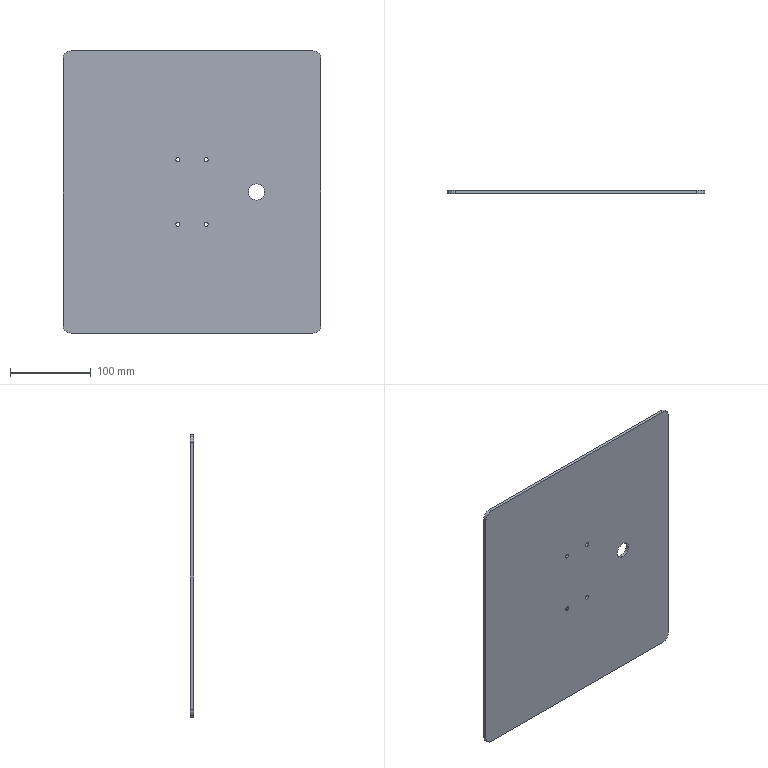Part | SolidWorks | features Extrusion 1, Fillet 1, HoleWzd 1, ICE 1 | 1 solid | 20 faces | box 320 x 4 x 350 mm | volume 446060 mm3 | cylinder 14 | plane 6 | commonest cylinder face diameters 5.2 x8 20 x6
STEP:
#1=CARTESIAN_POINT('',(80.,0.,-10.));
#2=VERTEX_POINT('',#1);
#3=CARTESIAN_POINT('',(80.,0.,10.));
#4=VERTEX_POINT('',#3);
#5=CARTESIAN_POINT('',(80.,0.,0.));
#6=DIRECTION('',(0.,1.,0.));
#7=DIRECTION('',(0.,0.,1.));
#8=AXIS2_PLACEMENT_3D('',#5,#6,#7);
#9=CIRCLE('',#8,10.);
#10=EDGE_CURVE('',#2,#4,#9,.T.);
#11=ORIENTED_EDGE('',*,*,#10,.F.);
#12=CARTESIAN_POINT('',(80.,4.,-10.));
#13=VERTEX_POINT('',#12);
#14=CARTESIAN_POINT('',(80.,0.,-10.));
#15=DIRECTION('',(0.,1.,0.));
#16=VECTOR('',#15,1000.);
#17=LINE('',#14,#16);
#18=EDGE_CURVE('',#2,#13,#17,.T.);
#19=ORIENTED_EDGE('',*,*,#18,.T.);
#20=CARTESIAN_POINT('',(80.,4.,10.));
#21=VERTEX_POINT('',#20);
#22=CARTESIAN_POINT('',(80.,4.,0.));
#23=DIRECTION('',(0.,1.,0.));
#24=DIRECTION('',(0.,0.,1.));
#25=AXIS2_PLACEMENT_3D('',#22,#23,#24);
#26=CIRCLE('',#25,10.);
#27=EDGE_CURVE('',#13,#21,#26,.T.);
#28=ORIENTED_EDGE('',*,*,#27,.T.);
#29=CARTESIAN_POINT('',(80.,0.,10.));
#30=DIRECTION('',(0.,1.,0.));
#31=VECTOR('',#30,1000.);
#32=LINE('',#29,#31);
#33=EDGE_CURVE('',#4,#21,#32,.T.);
#34=ORIENTED_EDGE('',*,*,#33,.F.);
#35=EDGE_LOOP('',(#11,#19,#28,#34));
#36=FACE_OUTER_BOUND('',#35,.T.);
#37=CARTESIAN_POINT('',(80.,0.,0.));
#38=DIRECTION('',(0.,1.,0.));
#39=DIRECTION('',(0.,0.,1.));
#40=AXIS2_PLACEMENT_3D('',#37,#38,#39);
#41=CYLINDRICAL_SURFACE('',#40,10.);
#42=ADVANCED_FACE('',(#36),#41,.F.);
#43=CARTESIAN_POINT('',(-17.5,0.,-42.6));
#44=VERTEX_POINT('',#43);
#45=CARTESIAN_POINT('',(-17.5,0.,-37.4));
#46=VERTEX_POINT('',#45);
#47=CARTESIAN_POINT('',(-17.5,0.,-40.));
#48=DIRECTION('',(0.,1.,0.));
#49=DIRECTION('',(0.,0.,1.));
#50=AXIS2_PLACEMENT_3D('',#47,#48,#49);
#51=CIRCLE('',#50,2.6);
#52=EDGE_CURVE('',#44,#46,#51,.T.);
#53=ORIENTED_EDGE('',*,*,#52,.F.);
#54=CARTESIAN_POINT('',(-17.5,4.,-42.6));
#55=VERTEX_POINT('',#54);
#56=CARTESIAN_POINT('',(-17.5,4.,-42.6));
#57=DIRECTION('',(0.,1.,0.));
#58=VECTOR('',#57,1000.);
#59=LINE('',#56,#58);
#60=EDGE_CURVE('',#44,#55,#59,.T.);
#61=ORIENTED_EDGE('',*,*,#60,.T.);
#62=CARTESIAN_POINT('',(-17.5,4.,-37.4));
#63=VERTEX_POINT('',#62);
#64=CARTESIAN_POINT('',(-17.5,4.,-40.));
#65=DIRECTION('',(0.,1.,0.));
#66=DIRECTION('',(0.,0.,1.));
#67=AXIS2_PLACEMENT_3D('',#64,#65,#66);
#68=CIRCLE('',#67,2.6);
#69=EDGE_CURVE('',#55,#63,#68,.T.);
#70=ORIENTED_EDGE('',*,*,#69,.T.);
#71=CARTESIAN_POINT('',(-17.5,4.,-37.4));
#72=DIRECTION('',(0.,1.,0.));
#73=VECTOR('',#72,1000.);
#74=LINE('',#71,#73);
#75=EDGE_CURVE('',#46,#63,#74,.T.);
#76=ORIENTED_EDGE('',*,*,#75,.F.);
#77=EDGE_LOOP('',(#53,#61,#70,#76));
#78=FACE_OUTER_BOUND('',#77,.T.);
#79=CARTESIAN_POINT('',(-17.5,4.,-40.));
#80=DIRECTION('',(0.,1.,0.));
#81=DIRECTION('',(0.,0.,1.));
#82=AXIS2_PLACEMENT_3D('',#79,#80,#81);
#83=CYLINDRICAL_SURFACE('',#82,2.6);
#84=ADVANCED_FACE('',(#78),#83,.F.);
#85=CARTESIAN_POINT('',(17.5,0.,37.4));
#86=VERTEX_POINT('',#85);
#87=CARTESIAN_POINT('',(17.5,0.,42.6));
#88=VERTEX_POINT('',#87);
#89=CARTESIAN_POINT('',(17.5,0.,40.));
#90=DIRECTION('',(0.,1.,0.));
#91=DIRECTION('',(0.,0.,1.));
#92=AXIS2_PLACEMENT_3D('',#89,#90,#91);
#93=CIRCLE('',#92,2.6);
#94=EDGE_CURVE('',#86,#88,#93,.T.);
#95=ORIENTED_EDGE('',*,*,#94,.F.);
#96=CARTESIAN_POINT('',(17.5,4.,37.4));
#97=VERTEX_POINT('',#96);
#98=CARTESIAN_POINT('',(17.5,4.,37.4));
#99=DIRECTION('',(0.,1.,0.));
#100=VECTOR('',#99,1000.);
#101=LINE('',#98,#100);
#102=EDGE_CURVE('',#86,#97,#101,.T.);
#103=ORIENTED_EDGE('',*,*,#102,.T.);
#104=CARTESIAN_POINT('',(17.5,4.,42.6));
#105=VERTEX_POINT('',#104);
#106=CARTESIAN_POINT('',(17.5,4.,40.));
#107=DIRECTION('',(0.,1.,0.));
#108=DIRECTION('',(0.,0.,1.));
#109=AXIS2_PLACEMENT_3D('',#106,#107,#108);
#110=CIRCLE('',#109,2.6);
#111=EDGE_CURVE('',#97,#105,#110,.T.);
#112=ORIENTED_EDGE('',*,*,#111,.T.);
#113=CARTESIAN_POINT('',(17.5,4.,42.6));
#114=DIRECTION('',(0.,1.,0.));
#115=VECTOR('',#114,1000.);
#116=LINE('',#113,#115);
#117=EDGE_CURVE('',#88,#105,#116,.T.);
#118=ORIENTED_EDGE('',*,*,#117,.F.);
#119=EDGE_LOOP('',(#95,#103,#112,#118));
#120=FACE_OUTER_BOUND('',#119,.T.);
#121=CARTESIAN_POINT('',(17.5,4.,40.));
#122=DIRECTION('',(0.,1.,0.));
#123=DIRECTION('',(0.,0.,1.));
#124=AXIS2_PLACEMENT_3D('',#121,#122,#123);
#125=CYLINDRICAL_SURFACE('',#124,2.6);
#126=ADVANCED_FACE('',(#120),#125,.F.);
#127=CARTESIAN_POINT('',(-17.5,0.,37.4));
#128=VERTEX_POINT('',#127);
#129=CARTESIAN_POINT('',(-17.5,0.,42.6));
#130=VERTEX_POINT('',#129);
#131=CARTESIAN_POINT('',(-17.5,0.,40.));
#132=DIRECTION('',(0.,1.,0.));
#133=DIRECTION('',(0.,0.,1.));
#134=AXIS2_PLACEMENT_3D('',#131,#132,#133);
#135=CIRCLE('',#134,2.6);
#136=EDGE_CURVE('',#128,#130,#135,.T.);
#137=ORIENTED_EDGE('',*,*,#136,.F.);
#138=CARTESIAN_POINT('',(-17.5,4.,37.4));
#139=VERTEX_POINT('',#138);
#140=CARTESIAN_POINT('',(-17.5,4.,37.4));
#141=DIRECTION('',(0.,1.,0.));
#142=VECTOR('',#141,1000.);
#143=LINE('',#140,#142);
#144=EDGE_CURVE('',#128,#139,#143,.T.);
#145=ORIENTED_EDGE('',*,*,#144,.T.);
#146=CARTESIAN_POINT('',(-17.5,4.,42.6));
#147=VERTEX_POINT('',#146);
#148=CARTESIAN_POINT('',(-17.5,4.,40.));
#149=DIRECTION('',(0.,1.,0.));
#150=DIRECTION('',(0.,0.,1.));
#151=AXIS2_PLACEMENT_3D('',#148,#149,#150);
#152=CIRCLE('',#151,2.6);
#153=EDGE_CURVE('',#139,#147,#152,.T.);
#154=ORIENTED_EDGE('',*,*,#153,.T.);
#155=CARTESIAN_POINT('',(-17.5,4.,42.6));
#156=DIRECTION('',(0.,1.,0.));
#157=VECTOR('',#156,1000.);
#158=LINE('',#155,#157);
#159=EDGE_CURVE('',#130,#147,#158,.T.);
#160=ORIENTED_EDGE('',*,*,#159,.F.);
#161=EDGE_LOOP('',(#137,#145,#154,#160));
#162=FACE_OUTER_BOUND('',#161,.T.);
#163=CARTESIAN_POINT('',(-17.5,4.,40.));
#164=DIRECTION('',(0.,1.,0.));
#165=DIRECTION('',(0.,0.,1.));
#166=AXIS2_PLACEMENT_3D('',#163,#164,#165);
#167=CYLINDRICAL_SURFACE('',#166,2.6);
#168=ADVANCED_FACE('',(#162),#167,.F.);
#169=CARTESIAN_POINT('',(17.5,0.,-42.6));
#170=VERTEX_POINT('',#169);
#171=CARTESIAN_POINT('',(17.5,0.,-37.4));
#172=VERTEX_POINT('',#171);
#173=CARTESIAN_POINT('',(17.5,0.,-40.));
#174=DIRECTION('',(0.,1.,0.));
#175=DIRECTION('',(0.,0.,1.));
#176=AXIS2_PLACEMENT_3D('',#173,#174,#175);
#177=CIRCLE('',#176,2.6);
#178=EDGE_CURVE('',#170,#172,#177,.T.);
#179=ORIENTED_EDGE('',*,*,#178,.F.);
#180=CARTESIAN_POINT('',(17.5,4.,-42.6));
#181=VERTEX_POINT('',#180);
#182=CARTESIAN_POINT('',(17.5,4.,-42.6));
#183=DIRECTION('',(0.,1.,0.));
#184=VECTOR('',#183,1000.);
#185=LINE('',#182,#184);
#186=EDGE_CURVE('',#170,#181,#185,.T.);
#187=ORIENTED_EDGE('',*,*,#186,.T.);
#188=CARTESIAN_POINT('',(17.5,4.,-37.4));
#189=VERTEX_POINT('',#188);
#190=CARTESIAN_POINT('',(17.5,4.,-40.));
#191=DIRECTION('',(0.,1.,0.));
#192=DIRECTION('',(0.,0.,1.));
#193=AXIS2_PLACEMENT_3D('',#190,#191,#192);
#194=CIRCLE('',#193,2.6);
#195=EDGE_CURVE('',#181,#189,#194,.T.);
#196=ORIENTED_EDGE('',*,*,#195,.T.);
#197=CARTESIAN_POINT('',(17.5,4.,-37.4));
#198=DIRECTION('',(0.,1.,0.));
#199=VECTOR('',#198,1000.);
#200=LINE('',#197,#199);
#201=EDGE_CURVE('',#172,#189,#200,.T.);
#202=ORIENTED_EDGE('',*,*,#201,.F.);
#203=EDGE_LOOP('',(#179,#187,#196,#202));
#204=FACE_OUTER_BOUND('',#203,.T.);
#205=CARTESIAN_POINT('',(17.5,4.,-40.));
#206=DIRECTION('',(0.,1.,0.));
#207=DIRECTION('',(0.,0.,1.));
#208=AXIS2_PLACEMENT_3D('',#205,#206,#207);
#209=CYLINDRICAL_SURFACE('',#208,2.6);
#210=ADVANCED_FACE('',(#204),#209,.F.);
#211=CARTESIAN_POINT('',(-160.,0.,-165.));
#212=VERTEX_POINT('',#211);
#213=CARTESIAN_POINT('',(-160.,0.,165.));
#214=VERTEX_POINT('',#213);
#215=CARTESIAN_POINT('',(-160.,0.,175.));
#216=DIRECTION('',(0.,0.,1.));
#217=VECTOR('',#216,1000.);
#218=LINE('',#215,#217);
#219=EDGE_CURVE('',#212,#214,#218,.T.);
#220=ORIENTED_EDGE('',*,*,#219,.T.);
#221=CARTESIAN_POINT('',(-160.,4.,165.));
#222=VERTEX_POINT('',#221);
#223=CARTESIAN_POINT('',(-160.,4.,165.));
#224=DIRECTION('',(0.,1.,0.));
#225=VECTOR('',#224,1000.);
#226=LINE('',#223,#225);
#227=EDGE_CURVE('',#214,#222,#226,.T.);
#228=ORIENTED_EDGE('',*,*,#227,.T.);
#229=CARTESIAN_POINT('',(-160.,4.,-165.));
#230=VERTEX_POINT('',#229);
#231=CARTESIAN_POINT('',(-160.,4.,175.));
#232=DIRECTION('',(0.,0.,1.));
#233=VECTOR('',#232,1000.);
#234=LINE('',#231,#233);
#235=EDGE_CURVE('',#230,#222,#234,.T.);
#236=ORIENTED_EDGE('',*,*,#235,.F.);
#237=CARTESIAN_POINT('',(-160.,4.,-165.));
#238=DIRECTION('',(0.,-1.,0.));
#239=VECTOR('',#238,1000.);
#240=LINE('',#237,#239);
#241=EDGE_CURVE('',#230,#212,#240,.T.);
#242=ORIENTED_EDGE('',*,*,#241,.T.);
#243=EDGE_LOOP('',(#220,#228,#236,#242));
#244=FACE_OUTER_BOUND('',#243,.T.);
#245=CARTESIAN_POINT('',(-160.,4.,175.));
#246=DIRECTION('',(1.,0.,0.));
#247=DIRECTION('',(0.,0.,-1.));
#248=AXIS2_PLACEMENT_3D('',#245,#246,#247);
#249=PLANE('',#248);
#250=ADVANCED_FACE('',(#244),#249,.F.);
#251=CARTESIAN_POINT('',(-150.,4.,175.));
#252=VERTEX_POINT('',#251);
#253=CARTESIAN_POINT('',(150.,4.,175.));
#254=VERTEX_POINT('',#253);
#255=CARTESIAN_POINT('',(160.,4.,175.));
#256=DIRECTION('',(1.,0.,0.));
#257=VECTOR('',#256,1000.);
#258=LINE('',#255,#257);
#259=EDGE_CURVE('',#252,#254,#258,.T.);
#260=ORIENTED_EDGE('',*,*,#259,.F.);
#261=CARTESIAN_POINT('',(-150.,0.,175.));
#262=VERTEX_POINT('',#261);
#263=CARTESIAN_POINT('',(-150.,4.,175.));
#264=DIRECTION('',(0.,-1.,0.));
#265=VECTOR('',#264,1000.);
#266=LINE('',#263,#265);
#267=EDGE_CURVE('',#252,#262,#266,.T.);
#268=ORIENTED_EDGE('',*,*,#267,.T.);
#269=CARTESIAN_POINT('',(150.,0.,175.));
#270=VERTEX_POINT('',#269);
#271=CARTESIAN_POINT('',(160.,0.,175.));
#272=DIRECTION('',(1.,0.,0.));
#273=VECTOR('',#272,1000.);
#274=LINE('',#271,#273);
#275=EDGE_CURVE('',#262,#270,#274,.T.);
#276=ORIENTED_EDGE('',*,*,#275,.T.);
#277=CARTESIAN_POINT('',(150.,4.,175.));
#278=DIRECTION('',(0.,1.,0.));
#279=VECTOR('',#278,1000.);
#280=LINE('',#277,#279);
#281=EDGE_CURVE('',#270,#254,#280,.T.);
#282=ORIENTED_EDGE('',*,*,#281,.T.);
#283=EDGE_LOOP('',(#260,#268,#276,#282));
#284=FACE_OUTER_BOUND('',#283,.T.);
#285=CARTESIAN_POINT('',(160.,4.,175.));
#286=DIRECTION('',(0.,0.,-1.));
#287=DIRECTION('',(-1.,0.,0.));
#288=AXIS2_PLACEMENT_3D('',#285,#286,#287);
#289=PLANE('',#288);
#290=ADVANCED_FACE('',(#284),#289,.F.);
#291=CARTESIAN_POINT('',(160.,4.,165.));
#292=VERTEX_POINT('',#291);
#293=CARTESIAN_POINT('',(160.,4.,-165.));
#294=VERTEX_POINT('',#293);
#295=CARTESIAN_POINT('',(160.,4.,175.));
#296=DIRECTION('',(0.,0.,-1.));
#297=VECTOR('',#296,1000.);
#298=LINE('',#295,#297);
#299=EDGE_CURVE('',#292,#294,#298,.T.);
#300=ORIENTED_EDGE('',*,*,#299,.F.);
#301=CARTESIAN_POINT('',(160.,0.,165.));
#302=VERTEX_POINT('',#301);
#303=CARTESIAN_POINT('',(160.,4.,165.));
#304=DIRECTION('',(0.,-1.,0.));
#305=VECTOR('',#304,1000.);
#306=LINE('',#303,#305);
#307=EDGE_CURVE('',#292,#302,#306,.T.);
#308=ORIENTED_EDGE('',*,*,#307,.T.);
#309=CARTESIAN_POINT('',(160.,0.,-165.));
#310=VERTEX_POINT('',#309);
#311=CARTESIAN_POINT('',(160.,0.,175.));
#312=DIRECTION('',(0.,0.,-1.));
#313=VECTOR('',#312,1000.);
#314=LINE('',#311,#313);
#315=EDGE_CURVE('',#302,#310,#314,.T.);
#316=ORIENTED_EDGE('',*,*,#315,.T.);
#317=CARTESIAN_POINT('',(160.,4.,-165.));
#318=DIRECTION('',(0.,1.,0.));
#319=VECTOR('',#318,1000.);
#320=LINE('',#317,#319);
#321=EDGE_CURVE('',#310,#294,#320,.T.);
#322=ORIENTED_EDGE('',*,*,#321,.T.);
#323=EDGE_LOOP('',(#300,#308,#316,#322));
#324=FACE_OUTER_BOUND('',#323,.T.);
#325=CARTESIAN_POINT('',(160.,4.,175.));
#326=DIRECTION('',(-1.,0.,0.));
#327=DIRECTION('',(0.,0.,1.));
#328=AXIS2_PLACEMENT_3D('',#325,#326,#327);
#329=PLANE('',#328);
#330=ADVANCED_FACE('',(#324),#329,.F.);
#331=CARTESIAN_POINT('',(150.,4.,-175.));
#332=VERTEX_POINT('',#331);
#333=CARTESIAN_POINT('',(-150.,4.,-175.));
#334=VERTEX_POINT('',#333);
#335=CARTESIAN_POINT('',(160.,4.,-175.));
#336=DIRECTION('',(-1.,0.,0.));
#337=VECTOR('',#336,1000.);
#338=LINE('',#335,#337);
#339=EDGE_CURVE('',#332,#334,#338,.T.);
#340=ORIENTED_EDGE('',*,*,#339,.F.);
#341=CARTESIAN_POINT('',(150.,0.,-175.));
#342=VERTEX_POINT('',#341);
#343=CARTESIAN_POINT('',(150.,4.,-175.));
#344=DIRECTION('',(0.,-1.,0.));
#345=VECTOR('',#344,1000.);
#346=LINE('',#343,#345);
#347=EDGE_CURVE('',#332,#342,#346,.T.);
#348=ORIENTED_EDGE('',*,*,#347,.T.);
#349=CARTESIAN_POINT('',(-150.,0.,-175.));
#350=VERTEX_POINT('',#349);
#351=CARTESIAN_POINT('',(160.,0.,-175.));
#352=DIRECTION('',(-1.,0.,0.));
#353=VECTOR('',#352,1000.);
#354=LINE('',#351,#353);
#355=EDGE_CURVE('',#342,#350,#354,.T.);
#356=ORIENTED_EDGE('',*,*,#355,.T.);
#357=CARTESIAN_POINT('',(-150.,4.,-175.));
#358=DIRECTION('',(0.,1.,0.));
#359=VECTOR('',#358,1000.);
#360=LINE('',#357,#359);
#361=EDGE_CURVE('',#350,#334,#360,.T.);
#362=ORIENTED_EDGE('',*,*,#361,.T.);
#363=EDGE_LOOP('',(#340,#348,#356,#362));
#364=FACE_OUTER_BOUND('',#363,.T.);
#365=CARTESIAN_POINT('',(160.,4.,-175.));
#366=DIRECTION('',(0.,0.,1.));
#367=DIRECTION('',(1.,0.,0.));
#368=AXIS2_PLACEMENT_3D('',#365,#366,#367);
#369=PLANE('',#368);
#370=ADVANCED_FACE('',(#364),#369,.F.);
#371=CARTESIAN_POINT('',(80.,4.,0.));
#372=DIRECTION('',(0.,1.,0.));
#373=DIRECTION('',(0.,0.,1.));
#374=AXIS2_PLACEMENT_3D('',#371,#372,#373);
#375=CIRCLE('',#374,10.);
#376=EDGE_CURVE('',#21,#13,#375,.T.);
#377=ORIENTED_EDGE('',*,*,#376,.F.);
#378=ORIENTED_EDGE('',*,*,#27,.F.);
#379=EDGE_LOOP('',(#377,#378));
#380=FACE_BOUND('',#379,.T.);
#381=CARTESIAN_POINT('',(-17.5,4.,-40.));
#382=DIRECTION('',(0.,1.,0.));
#383=DIRECTION('',(0.,0.,1.));
#384=AXIS2_PLACEMENT_3D('',#381,#382,#383);
#385=CIRCLE('',#384,2.6);
#386=EDGE_CURVE('',#63,#55,#385,.T.);
#387=ORIENTED_EDGE('',*,*,#386,.F.);
#388=ORIENTED_EDGE('',*,*,#69,.F.);
#389=EDGE_LOOP('',(#387,#388));
#390=FACE_BOUND('',#389,.T.);
#391=CARTESIAN_POINT('',(17.5,4.,40.));
#392=DIRECTION('',(0.,1.,0.));
#393=DIRECTION('',(0.,0.,1.));
#394=AXIS2_PLACEMENT_3D('',#391,#392,#393);
#395=CIRCLE('',#394,2.6);
#396=EDGE_CURVE('',#105,#97,#395,.T.);
#397=ORIENTED_EDGE('',*,*,#396,.F.);
#398=ORIENTED_EDGE('',*,*,#111,.F.);
#399=EDGE_LOOP('',(#397,#398));
#400=FACE_BOUND('',#399,.T.);
#401=CARTESIAN_POINT('',(-17.5,4.,40.));
#402=DIRECTION('',(0.,1.,0.));
#403=DIRECTION('',(0.,0.,1.));
#404=AXIS2_PLACEMENT_3D('',#401,#402,#403);
#405=CIRCLE('',#404,2.6);
#406=EDGE_CURVE('',#147,#139,#405,.T.);
#407=ORIENTED_EDGE('',*,*,#406,.F.);
#408=ORIENTED_EDGE('',*,*,#153,.F.);
#409=EDGE_LOOP('',(#407,#408));
#410=FACE_BOUND('',#409,.T.);
#411=CARTESIAN_POINT('',(17.5,4.,-40.));
#412=DIRECTION('',(0.,1.,0.));
#413=DIRECTION('',(0.,0.,1.));
#414=AXIS2_PLACEMENT_3D('',#411,#412,#413);
#415=CIRCLE('',#414,2.6);
#416=EDGE_CURVE('',#189,#181,#415,.T.);
#417=ORIENTED_EDGE('',*,*,#416,.F.);
#418=ORIENTED_EDGE('',*,*,#195,.F.);
#419=EDGE_LOOP('',(#417,#418));
#420=FACE_BOUND('',#419,.T.);
#421=ORIENTED_EDGE('',*,*,#235,.T.);
#422=CARTESIAN_POINT('',(-150.,4.,165.));
#423=DIRECTION('',(0.,1.,0.));
#424=DIRECTION('',(0.,0.,1.));
#425=AXIS2_PLACEMENT_3D('',#422,#423,#424);
#426=CIRCLE('',#425,10.);
#427=EDGE_CURVE('',#222,#252,#426,.T.);
#428=ORIENTED_EDGE('',*,*,#427,.T.);
#429=ORIENTED_EDGE('',*,*,#259,.T.);
#430=CARTESIAN_POINT('',(150.,4.,165.));
#431=DIRECTION('',(0.,1.,0.));
#432=DIRECTION('',(0.,0.,1.));
#433=AXIS2_PLACEMENT_3D('',#430,#431,#432);
#434=CIRCLE('',#433,10.);
#435=EDGE_CURVE('',#254,#292,#434,.T.);
#436=ORIENTED_EDGE('',*,*,#435,.T.);
#437=ORIENTED_EDGE('',*,*,#299,.T.);
#438=CARTESIAN_POINT('',(150.,4.,-165.));
#439=DIRECTION('',(0.,1.,0.));
#440=DIRECTION('',(0.,0.,1.));
#441=AXIS2_PLACEMENT_3D('',#438,#439,#440);
#442=CIRCLE('',#441,10.);
#443=EDGE_CURVE('',#294,#332,#442,.T.);
#444=ORIENTED_EDGE('',*,*,#443,.T.);
#445=ORIENTED_EDGE('',*,*,#339,.T.);
#446=CARTESIAN_POINT('',(-150.,4.,-165.));
#447=DIRECTION('',(0.,1.,0.));
#448=DIRECTION('',(0.,0.,1.));
#449=AXIS2_PLACEMENT_3D('',#446,#447,#448);
#450=CIRCLE('',#449,10.);
#451=EDGE_CURVE('',#334,#230,#450,.T.);
#452=ORIENTED_EDGE('',*,*,#451,.T.);
#453=EDGE_LOOP('',(#421,#428,#429,#436,#437,#444,#445,#452));
#454=FACE_OUTER_BOUND('',#453,.T.);
#455=CARTESIAN_POINT('',(0.,4.,0.));
#456=DIRECTION('',(0.,1.,0.));
#457=DIRECTION('',(0.,0.,1.));
#458=AXIS2_PLACEMENT_3D('',#455,#456,#457);
#459=PLANE('',#458);
#460=ADVANCED_FACE('',(#380,#390,#400,#410,#420,#454),#459,.T.);
#461=CARTESIAN_POINT('',(80.,0.,0.));
#462=DIRECTION('',(0.,1.,0.));
#463=DIRECTION('',(0.,0.,1.));
#464=AXIS2_PLACEMENT_3D('',#461,#462,#463);
#465=CIRCLE('',#464,10.);
#466=EDGE_CURVE('',#4,#2,#465,.T.);
#467=ORIENTED_EDGE('',*,*,#466,.T.);
#468=ORIENTED_EDGE('',*,*,#10,.T.);
#469=EDGE_LOOP('',(#467,#468));
#470=FACE_BOUND('',#469,.T.);
#471=CARTESIAN_POINT('',(-17.5,0.,-40.));
#472=DIRECTION('',(0.,1.,0.));
#473=DIRECTION('',(0.,0.,1.));
#474=AXIS2_PLACEMENT_3D('',#471,#472,#473);
#475=CIRCLE('',#474,2.6);
#476=EDGE_CURVE('',#46,#44,#475,.T.);
#477=ORIENTED_EDGE('',*,*,#476,.T.);
#478=ORIENTED_EDGE('',*,*,#52,.T.);
#479=EDGE_LOOP('',(#477,#478));
#480=FACE_BOUND('',#479,.T.);
#481=CARTESIAN_POINT('',(17.5,0.,40.));
#482=DIRECTION('',(0.,1.,0.));
#483=DIRECTION('',(0.,0.,1.));
#484=AXIS2_PLACEMENT_3D('',#481,#482,#483);
#485=CIRCLE('',#484,2.6);
#486=EDGE_CURVE('',#88,#86,#485,.T.);
#487=ORIENTED_EDGE('',*,*,#486,.T.);
#488=ORIENTED_EDGE('',*,*,#94,.T.);
#489=EDGE_LOOP('',(#487,#488));
#490=FACE_BOUND('',#489,.T.);
#491=CARTESIAN_POINT('',(-17.5,0.,40.));
#492=DIRECTION('',(0.,1.,0.));
#493=DIRECTION('',(0.,0.,1.));
#494=AXIS2_PLACEMENT_3D('',#491,#492,#493);
#495=CIRCLE('',#494,2.6);
#496=EDGE_CURVE('',#130,#128,#495,.T.);
#497=ORIENTED_EDGE('',*,*,#496,.T.);
#498=ORIENTED_EDGE('',*,*,#136,.T.);
#499=EDGE_LOOP('',(#497,#498));
#500=FACE_BOUND('',#499,.T.);
#501=CARTESIAN_POINT('',(17.5,0.,-40.));
#502=DIRECTION('',(0.,1.,0.));
#503=DIRECTION('',(0.,0.,1.));
#504=AXIS2_PLACEMENT_3D('',#501,#502,#503);
#505=CIRCLE('',#504,2.6);
#506=EDGE_CURVE('',#172,#170,#505,.T.);
#507=ORIENTED_EDGE('',*,*,#506,.T.);
#508=ORIENTED_EDGE('',*,*,#178,.T.);
#509=EDGE_LOOP('',(#507,#508));
#510=FACE_BOUND('',#509,.T.);
#511=ORIENTED_EDGE('',*,*,#275,.F.);
#512=CARTESIAN_POINT('',(-150.,0.,165.));
#513=DIRECTION('',(0.,-1.,0.));
#514=DIRECTION('',(0.,0.,1.));
#515=AXIS2_PLACEMENT_3D('',#512,#513,#514);
#516=CIRCLE('',#515,10.);
#517=EDGE_CURVE('',#262,#214,#516,.T.);
#518=ORIENTED_EDGE('',*,*,#517,.T.);
#519=ORIENTED_EDGE('',*,*,#219,.F.);
#520=CARTESIAN_POINT('',(-150.,0.,-165.));
#521=DIRECTION('',(0.,-1.,0.));
#522=DIRECTION('',(0.,0.,1.));
#523=AXIS2_PLACEMENT_3D('',#520,#521,#522);
#524=CIRCLE('',#523,10.);
#525=EDGE_CURVE('',#212,#350,#524,.T.);
#526=ORIENTED_EDGE('',*,*,#525,.T.);
#527=ORIENTED_EDGE('',*,*,#355,.F.);
#528=CARTESIAN_POINT('',(150.,0.,-165.));
#529=DIRECTION('',(0.,-1.,0.));
#530=DIRECTION('',(0.,0.,1.));
#531=AXIS2_PLACEMENT_3D('',#528,#529,#530);
#532=CIRCLE('',#531,10.);
#533=EDGE_CURVE('',#342,#310,#532,.T.);
#534=ORIENTED_EDGE('',*,*,#533,.T.);
#535=ORIENTED_EDGE('',*,*,#315,.F.);
#536=CARTESIAN_POINT('',(150.,0.,165.));
#537=DIRECTION('',(0.,-1.,0.));
#538=DIRECTION('',(0.,0.,1.));
#539=AXIS2_PLACEMENT_3D('',#536,#537,#538);
#540=CIRCLE('',#539,10.);
#541=EDGE_CURVE('',#302,#270,#540,.T.);
#542=ORIENTED_EDGE('',*,*,#541,.T.);
#543=EDGE_LOOP('',(#511,#518,#519,#526,#527,#534,#535,#542));
#544=FACE_OUTER_BOUND('',#543,.T.);
#545=CARTESIAN_POINT('',(0.,0.,0.));
#546=DIRECTION('',(0.,1.,0.));
#547=DIRECTION('',(0.,0.,1.));
#548=AXIS2_PLACEMENT_3D('',#545,#546,#547);
#549=PLANE('',#548);
#550=ADVANCED_FACE('',(#470,#480,#490,#500,#510,#544),#549,.F.);
#551=ORIENTED_EDGE('',*,*,#186,.F.);
#552=ORIENTED_EDGE('',*,*,#506,.F.);
#553=ORIENTED_EDGE('',*,*,#201,.T.);
#554=ORIENTED_EDGE('',*,*,#416,.T.);
#555=EDGE_LOOP('',(#551,#552,#553,#554));
#556=FACE_OUTER_BOUND('',#555,.T.);
#557=CARTESIAN_POINT('',(17.5,4.,-40.));
#558=DIRECTION('',(0.,1.,0.));
#559=DIRECTION('',(0.,0.,1.));
#560=AXIS2_PLACEMENT_3D('',#557,#558,#559);
#561=CYLINDRICAL_SURFACE('',#560,2.6);
#562=ADVANCED_FACE('',(#556),#561,.F.);
#563=ORIENTED_EDGE('',*,*,#144,.F.);
#564=ORIENTED_EDGE('',*,*,#496,.F.);
#565=ORIENTED_EDGE('',*,*,#159,.T.);
#566=ORIENTED_EDGE('',*,*,#406,.T.);
#567=EDGE_LOOP('',(#563,#564,#565,#566));
#568=FACE_OUTER_BOUND('',#567,.T.);
#569=CARTESIAN_POINT('',(-17.5,4.,40.));
#570=DIRECTION('',(0.,1.,0.));
#571=DIRECTION('',(0.,0.,1.));
#572=AXIS2_PLACEMENT_3D('',#569,#570,#571);
#573=CYLINDRICAL_SURFACE('',#572,2.6);
#574=ADVANCED_FACE('',(#568),#573,.F.);
#575=ORIENTED_EDGE('',*,*,#102,.F.);
#576=ORIENTED_EDGE('',*,*,#486,.F.);
#577=ORIENTED_EDGE('',*,*,#117,.T.);
#578=ORIENTED_EDGE('',*,*,#396,.T.);
#579=EDGE_LOOP('',(#575,#576,#577,#578));
#580=FACE_OUTER_BOUND('',#579,.T.);
#581=CARTESIAN_POINT('',(17.5,4.,40.));
#582=DIRECTION('',(0.,1.,0.));
#583=DIRECTION('',(0.,0.,1.));
#584=AXIS2_PLACEMENT_3D('',#581,#582,#583);
#585=CYLINDRICAL_SURFACE('',#584,2.6);
#586=ADVANCED_FACE('',(#580),#585,.F.);
#587=ORIENTED_EDGE('',*,*,#60,.F.);
#588=ORIENTED_EDGE('',*,*,#476,.F.);
#589=ORIENTED_EDGE('',*,*,#75,.T.);
#590=ORIENTED_EDGE('',*,*,#386,.T.);
#591=EDGE_LOOP('',(#587,#588,#589,#590));
#592=FACE_OUTER_BOUND('',#591,.T.);
#593=CARTESIAN_POINT('',(-17.5,4.,-40.));
#594=DIRECTION('',(0.,1.,0.));
#595=DIRECTION('',(0.,0.,1.));
#596=AXIS2_PLACEMENT_3D('',#593,#594,#595);
#597=CYLINDRICAL_SURFACE('',#596,2.6);
#598=ADVANCED_FACE('',(#592),#597,.F.);
#599=ORIENTED_EDGE('',*,*,#427,.F.);
#600=ORIENTED_EDGE('',*,*,#227,.F.);
#601=ORIENTED_EDGE('',*,*,#517,.F.);
#602=ORIENTED_EDGE('',*,*,#267,.F.);
#603=EDGE_LOOP('',(#599,#600,#601,#602));
#604=FACE_OUTER_BOUND('',#603,.T.);
#605=CARTESIAN_POINT('',(-150.,4.,165.));
#606=DIRECTION('',(0.,-1.,0.));
#607=DIRECTION('',(0.,0.,-1.));
#608=AXIS2_PLACEMENT_3D('',#605,#606,#607);
#609=CYLINDRICAL_SURFACE('',#608,10.);
#610=ADVANCED_FACE('',(#604),#609,.T.);
#611=ORIENTED_EDGE('',*,*,#435,.F.);
#612=ORIENTED_EDGE('',*,*,#281,.F.);
#613=ORIENTED_EDGE('',*,*,#541,.F.);
#614=ORIENTED_EDGE('',*,*,#307,.F.);
#615=EDGE_LOOP('',(#611,#612,#613,#614));
#616=FACE_OUTER_BOUND('',#615,.T.);
#617=CARTESIAN_POINT('',(150.,4.,165.));
#618=DIRECTION('',(0.,-1.,0.));
#619=DIRECTION('',(0.,0.,-1.));
#620=AXIS2_PLACEMENT_3D('',#617,#618,#619);
#621=CYLINDRICAL_SURFACE('',#620,10.);
#622=ADVANCED_FACE('',(#616),#621,.T.);
#623=ORIENTED_EDGE('',*,*,#443,.F.);
#624=ORIENTED_EDGE('',*,*,#321,.F.);
#625=ORIENTED_EDGE('',*,*,#533,.F.);
#626=ORIENTED_EDGE('',*,*,#347,.F.);
#627=EDGE_LOOP('',(#623,#624,#625,#626));
#628=FACE_OUTER_BOUND('',#627,.T.);
#629=CARTESIAN_POINT('',(150.,4.,-165.));
#630=DIRECTION('',(0.,-1.,0.));
#631=DIRECTION('',(0.,0.,-1.));
#632=AXIS2_PLACEMENT_3D('',#629,#630,#631);
#633=CYLINDRICAL_SURFACE('',#632,10.);
#634=ADVANCED_FACE('',(#628),#633,.T.);
#635=ORIENTED_EDGE('',*,*,#451,.F.);
#636=ORIENTED_EDGE('',*,*,#361,.F.);
#637=ORIENTED_EDGE('',*,*,#525,.F.);
#638=ORIENTED_EDGE('',*,*,#241,.F.);
#639=EDGE_LOOP('',(#635,#636,#637,#638));
#640=FACE_OUTER_BOUND('',#639,.T.);
#641=CARTESIAN_POINT('',(-150.,4.,-165.));
#642=DIRECTION('',(0.,-1.,0.));
#643=DIRECTION('',(0.,0.,-1.));
#644=AXIS2_PLACEMENT_3D('',#641,#642,#643);
#645=CYLINDRICAL_SURFACE('',#644,10.);
#646=ADVANCED_FACE('',(#640),#645,.T.);
#647=ORIENTED_EDGE('',*,*,#18,.F.);
#648=ORIENTED_EDGE('',*,*,#466,.F.);
#649=ORIENTED_EDGE('',*,*,#33,.T.);
#650=ORIENTED_EDGE('',*,*,#376,.T.);
#651=EDGE_LOOP('',(#647,#648,#649,#650));
#652=FACE_OUTER_BOUND('',#651,.T.);
#653=CARTESIAN_POINT('',(80.,0.,0.));
#654=DIRECTION('',(0.,1.,0.));
#655=DIRECTION('',(0.,0.,1.));
#656=AXIS2_PLACEMENT_3D('',#653,#654,#655);
#657=CYLINDRICAL_SURFACE('',#656,10.);
#658=ADVANCED_FACE('',(#652),#657,.F.);
#659=CLOSED_SHELL('',(#42,#84,#126,#168,#210,#250,#290,#330,#370,#460,#550,#562,#574,#586,#598,#610,#622,#634,#646,#658));
#660=MANIFOLD_SOLID_BREP('',#659);
#661=CARTESIAN_POINT('',(0.,0.,0.));
#662=DIRECTION('',(0.,0.,1.));
#663=DIRECTION('',(1.,0.,0.));
#664=AXIS2_PLACEMENT_3D('',#661,#662,#663);
#665=(LENGTH_UNIT()NAMED_UNIT(*)SI_UNIT(.MILLI.,.METRE.));
#666=UNCERTAINTY_MEASURE_WITH_UNIT(LENGTH_MEASURE(0.00001),#665,'','');
#667=(NAMED_UNIT(*)PLANE_ANGLE_UNIT()SI_UNIT($,.RADIAN.));
#668=(NAMED_UNIT(*)SI_UNIT($,.STERADIAN.)SOLID_ANGLE_UNIT());
#669=(GEOMETRIC_REPRESENTATION_CONTEXT(3)GLOBAL_UNCERTAINTY_ASSIGNED_CONTEXT((#666))GLOBAL_UNIT_ASSIGNED_CONTEXT((#665,#667,#668))REPRESENTATION_CONTEXT('',''));
#670=ADVANCED_BREP_SHAPE_REPRESENTATION('',(#660,#664),#669);